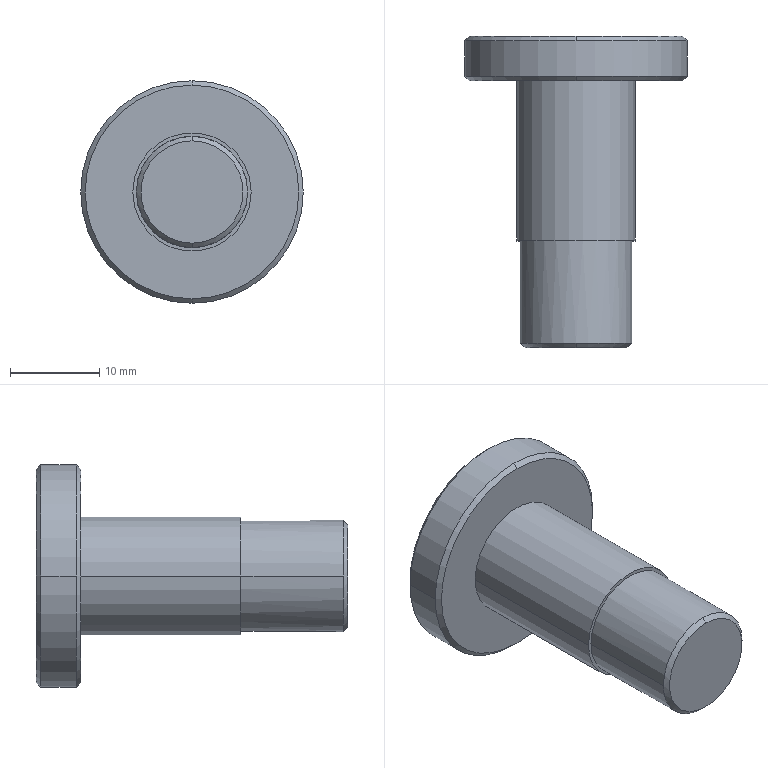Part | SolidWorks | features Chamfer 1, Revolution 1 | 1 solid | 16 faces | box 25 x 35 x 25 mm | volume 6404 mm3 | cone 6 | cylinder 6 | plane 4 | commonest cylinder face diameters 12.5 x2 13.3 x2 25 x2
STEP:
#1=CARTESIAN_POINT('',(-133.037,-447.686,-5.75));
#2=VERTEX_POINT('',#1);
#3=CARTESIAN_POINT('',(-133.037,-447.686,5.75));
#4=VERTEX_POINT('',#3);
#5=CARTESIAN_POINT('',(-133.037,-447.686,0.));
#6=DIRECTION('',(0.,-1.,0.));
#7=DIRECTION('',(1.,0.,0.));
#8=AXIS2_PLACEMENT_3D('',#5,#6,#7);
#9=CIRCLE('',#8,5.75);
#10=EDGE_CURVE('',#2,#4,#9,.T.);
#11=ORIENTED_EDGE('',*,*,#10,.F.);
#12=CARTESIAN_POINT('',(-133.037,-447.186,-6.25));
#13=VERTEX_POINT('',#12);
#14=CARTESIAN_POINT('',(-133.037,-447.186,-6.25));
#15=DIRECTION('',(0.,0.7071,-0.7071));
#16=VECTOR('',#15,1000.);
#17=LINE('',#14,#16);
#18=EDGE_CURVE('',#2,#13,#17,.T.);
#19=ORIENTED_EDGE('',*,*,#18,.T.);
#20=CARTESIAN_POINT('',(-126.787,-447.186,0.));
#21=VERTEX_POINT('',#20);
#22=CARTESIAN_POINT('',(-133.037,-447.186,0.));
#23=DIRECTION('',(0.,1.,0.));
#24=DIRECTION('',(0.,0.,-1.));
#25=AXIS2_PLACEMENT_3D('',#22,#23,#24);
#26=CIRCLE('',#25,6.25);
#27=EDGE_CURVE('',#21,#13,#26,.T.);
#28=ORIENTED_EDGE('',*,*,#27,.F.);
#29=CARTESIAN_POINT('',(-133.037,-447.186,6.25));
#30=VERTEX_POINT('',#29);
#31=CARTESIAN_POINT('',(-133.037,-447.186,0.));
#32=DIRECTION('',(0.,1.,0.));
#33=DIRECTION('',(0.,0.,-1.));
#34=AXIS2_PLACEMENT_3D('',#31,#32,#33);
#35=CIRCLE('',#34,6.25);
#36=EDGE_CURVE('',#30,#21,#35,.T.);
#37=ORIENTED_EDGE('',*,*,#36,.F.);
#38=CARTESIAN_POINT('',(-133.037,-447.186,6.25));
#39=DIRECTION('',(0.,0.7071,0.7071));
#40=VECTOR('',#39,1000.);
#41=LINE('',#38,#40);
#42=EDGE_CURVE('',#4,#30,#41,.T.);
#43=ORIENTED_EDGE('',*,*,#42,.F.);
#44=EDGE_LOOP('',(#11,#19,#28,#37,#43));
#45=FACE_OUTER_BOUND('',#44,.T.);
#46=CARTESIAN_POINT('',(-133.037,-447.186,0.));
#47=DIRECTION('',(0.,1.,0.));
#48=DIRECTION('',(0.,0.,1.));
#49=AXIS2_PLACEMENT_3D('',#46,#47,#48);
#50=CONICAL_SURFACE('',#49,6.25,0.7854);
#51=ADVANCED_FACE('',(#45),#50,.T.);
#52=CARTESIAN_POINT('',(-133.037,-417.686,-12.));
#53=VERTEX_POINT('',#52);
#54=CARTESIAN_POINT('',(-133.037,-417.686,12.));
#55=VERTEX_POINT('',#54);
#56=CARTESIAN_POINT('',(-133.037,-417.686,0.));
#57=DIRECTION('',(0.,-1.,0.));
#58=DIRECTION('',(1.,0.,0.));
#59=AXIS2_PLACEMENT_3D('',#56,#57,#58);
#60=CIRCLE('',#59,12.);
#61=EDGE_CURVE('',#53,#55,#60,.T.);
#62=ORIENTED_EDGE('',*,*,#61,.F.);
#63=CARTESIAN_POINT('',(-133.037,-417.186,-12.5));
#64=VERTEX_POINT('',#63);
#65=CARTESIAN_POINT('',(-133.037,-417.186,-12.5));
#66=DIRECTION('',(0.,0.7071,-0.7071));
#67=VECTOR('',#66,1000.);
#68=LINE('',#65,#67);
#69=EDGE_CURVE('',#53,#64,#68,.T.);
#70=ORIENTED_EDGE('',*,*,#69,.T.);
#71=CARTESIAN_POINT('',(-120.537,-417.186,0.));
#72=VERTEX_POINT('',#71);
#73=CARTESIAN_POINT('',(-133.037,-417.186,0.));
#74=DIRECTION('',(0.,1.,0.));
#75=DIRECTION('',(0.,0.,-1.));
#76=AXIS2_PLACEMENT_3D('',#73,#74,#75);
#77=CIRCLE('',#76,12.5);
#78=EDGE_CURVE('',#72,#64,#77,.T.);
#79=ORIENTED_EDGE('',*,*,#78,.F.);
#80=CARTESIAN_POINT('',(-133.037,-417.186,12.5));
#81=VERTEX_POINT('',#80);
#82=CARTESIAN_POINT('',(-133.037,-417.186,0.));
#83=DIRECTION('',(0.,1.,0.));
#84=DIRECTION('',(0.,0.,-1.));
#85=AXIS2_PLACEMENT_3D('',#82,#83,#84);
#86=CIRCLE('',#85,12.5);
#87=EDGE_CURVE('',#81,#72,#86,.T.);
#88=ORIENTED_EDGE('',*,*,#87,.F.);
#89=CARTESIAN_POINT('',(-133.037,-417.186,12.5));
#90=DIRECTION('',(0.,0.7071,0.7071));
#91=VECTOR('',#90,1000.);
#92=LINE('',#89,#91);
#93=EDGE_CURVE('',#55,#81,#92,.T.);
#94=ORIENTED_EDGE('',*,*,#93,.F.);
#95=EDGE_LOOP('',(#62,#70,#79,#88,#94));
#96=FACE_OUTER_BOUND('',#95,.T.);
#97=CARTESIAN_POINT('',(-133.037,-417.186,0.));
#98=DIRECTION('',(0.,1.,0.));
#99=DIRECTION('',(0.,0.,1.));
#100=AXIS2_PLACEMENT_3D('',#97,#98,#99);
#101=CONICAL_SURFACE('',#100,12.5,0.7854);
#102=ADVANCED_FACE('',(#96),#101,.T.);
#103=CARTESIAN_POINT('',(-133.037,-412.686,12.));
#104=VERTEX_POINT('',#103);
#105=CARTESIAN_POINT('',(-133.037,-412.686,-12.));
#106=VERTEX_POINT('',#105);
#107=CARTESIAN_POINT('',(-133.037,-412.686,0.));
#108=DIRECTION('',(0.,1.,0.));
#109=DIRECTION('',(-1.,0.,0.));
#110=AXIS2_PLACEMENT_3D('',#107,#108,#109);
#111=CIRCLE('',#110,12.);
#112=EDGE_CURVE('',#104,#106,#111,.T.);
#113=ORIENTED_EDGE('',*,*,#112,.F.);
#114=CARTESIAN_POINT('',(-133.037,-413.186,12.5));
#115=VERTEX_POINT('',#114);
#116=CARTESIAN_POINT('',(-133.037,-412.686,12.));
#117=DIRECTION('',(0.,-0.7071,0.7071));
#118=VECTOR('',#117,1000.);
#119=LINE('',#116,#118);
#120=EDGE_CURVE('',#104,#115,#119,.T.);
#121=ORIENTED_EDGE('',*,*,#120,.T.);
#122=CARTESIAN_POINT('',(-120.537,-413.186,0.));
#123=VERTEX_POINT('',#122);
#124=CARTESIAN_POINT('',(-133.037,-413.186,0.));
#125=DIRECTION('',(0.,-1.,0.));
#126=DIRECTION('',(0.,0.,1.));
#127=AXIS2_PLACEMENT_3D('',#124,#125,#126);
#128=CIRCLE('',#127,12.5);
#129=EDGE_CURVE('',#123,#115,#128,.T.);
#130=ORIENTED_EDGE('',*,*,#129,.F.);
#131=CARTESIAN_POINT('',(-133.037,-413.186,-12.5));
#132=VERTEX_POINT('',#131);
#133=CARTESIAN_POINT('',(-133.037,-413.186,0.));
#134=DIRECTION('',(0.,-1.,0.));
#135=DIRECTION('',(0.,0.,1.));
#136=AXIS2_PLACEMENT_3D('',#133,#134,#135);
#137=CIRCLE('',#136,12.5);
#138=EDGE_CURVE('',#132,#123,#137,.T.);
#139=ORIENTED_EDGE('',*,*,#138,.F.);
#140=CARTESIAN_POINT('',(-133.037,-412.686,-12.));
#141=DIRECTION('',(0.,-0.7071,-0.7071));
#142=VECTOR('',#141,1000.);
#143=LINE('',#140,#142);
#144=EDGE_CURVE('',#106,#132,#143,.T.);
#145=ORIENTED_EDGE('',*,*,#144,.F.);
#146=EDGE_LOOP('',(#113,#121,#130,#139,#145));
#147=FACE_OUTER_BOUND('',#146,.T.);
#148=CARTESIAN_POINT('',(-133.037,-412.686,0.));
#149=DIRECTION('',(0.,-1.,0.));
#150=DIRECTION('',(0.,0.,-1.));
#151=AXIS2_PLACEMENT_3D('',#148,#149,#150);
#152=CONICAL_SURFACE('',#151,12.,0.7854);
#153=ADVANCED_FACE('',(#147),#152,.T.);
#154=CARTESIAN_POINT('',(-145.537,-417.186,0.));
#155=VERTEX_POINT('',#154);
#156=CARTESIAN_POINT('',(-133.037,-417.186,0.));
#157=DIRECTION('',(0.,1.,0.));
#158=DIRECTION('',(0.,0.,-1.));
#159=AXIS2_PLACEMENT_3D('',#156,#157,#158);
#160=CIRCLE('',#159,12.5);
#161=EDGE_CURVE('',#155,#81,#160,.T.);
#162=ORIENTED_EDGE('',*,*,#161,.T.);
#163=ORIENTED_EDGE('',*,*,#87,.T.);
#164=CARTESIAN_POINT('',(-120.537,-412.686,0.));
#165=DIRECTION('',(0.,1.,0.));
#166=VECTOR('',#165,1000.);
#167=LINE('',#164,#166);
#168=EDGE_CURVE('',#72,#123,#167,.T.);
#169=ORIENTED_EDGE('',*,*,#168,.T.);
#170=ORIENTED_EDGE('',*,*,#129,.T.);
#171=CARTESIAN_POINT('',(-145.537,-413.186,0.));
#172=VERTEX_POINT('',#171);
#173=CARTESIAN_POINT('',(-133.037,-413.186,0.));
#174=DIRECTION('',(0.,-1.,0.));
#175=DIRECTION('',(0.,0.,1.));
#176=AXIS2_PLACEMENT_3D('',#173,#174,#175);
#177=CIRCLE('',#176,12.5);
#178=EDGE_CURVE('',#115,#172,#177,.T.);
#179=ORIENTED_EDGE('',*,*,#178,.T.);
#180=CARTESIAN_POINT('',(-145.537,-412.686,0.));
#181=DIRECTION('',(0.,1.,0.));
#182=VECTOR('',#181,1000.);
#183=LINE('',#180,#182);
#184=EDGE_CURVE('',#155,#172,#183,.T.);
#185=ORIENTED_EDGE('',*,*,#184,.F.);
#186=EDGE_LOOP('',(#162,#163,#169,#170,#179,#185));
#187=FACE_OUTER_BOUND('',#186,.T.);
#188=CARTESIAN_POINT('',(-133.037,-412.686,0.));
#189=DIRECTION('',(0.,1.,0.));
#190=DIRECTION('',(-1.,0.,0.));
#191=AXIS2_PLACEMENT_3D('',#188,#189,#190);
#192=CYLINDRICAL_SURFACE('',#191,12.5);
#193=ADVANCED_FACE('',(#187),#192,.T.);
#194=CARTESIAN_POINT('',(-139.687,-435.686,0.));
#195=VERTEX_POINT('',#194);
#196=CARTESIAN_POINT('',(-126.387,-435.686,0.));
#197=VERTEX_POINT('',#196);
#198=CARTESIAN_POINT('',(-133.037,-435.686,0.));
#199=DIRECTION('',(0.,1.,0.));
#200=DIRECTION('',(-1.,0.,0.));
#201=AXIS2_PLACEMENT_3D('',#198,#199,#200);
#202=CIRCLE('',#201,6.65);
#203=EDGE_CURVE('',#195,#197,#202,.T.);
#204=ORIENTED_EDGE('',*,*,#203,.T.);
#205=CARTESIAN_POINT('',(-126.387,-417.686,0.));
#206=VERTEX_POINT('',#205);
#207=CARTESIAN_POINT('',(-126.387,-412.686,0.));
#208=DIRECTION('',(0.,1.,0.));
#209=VECTOR('',#208,1000.);
#210=LINE('',#207,#209);
#211=EDGE_CURVE('',#197,#206,#210,.T.);
#212=ORIENTED_EDGE('',*,*,#211,.T.);
#213=CARTESIAN_POINT('',(-139.687,-417.686,0.));
#214=VERTEX_POINT('',#213);
#215=CARTESIAN_POINT('',(-133.037,-417.686,0.));
#216=DIRECTION('',(0.,1.,0.));
#217=DIRECTION('',(-1.,0.,0.));
#218=AXIS2_PLACEMENT_3D('',#215,#216,#217);
#219=CIRCLE('',#218,6.65);
#220=EDGE_CURVE('',#214,#206,#219,.T.);
#221=ORIENTED_EDGE('',*,*,#220,.F.);
#222=CARTESIAN_POINT('',(-139.687,-412.686,0.));
#223=DIRECTION('',(0.,1.,0.));
#224=VECTOR('',#223,1000.);
#225=LINE('',#222,#224);
#226=EDGE_CURVE('',#195,#214,#225,.T.);
#227=ORIENTED_EDGE('',*,*,#226,.F.);
#228=EDGE_LOOP('',(#204,#212,#221,#227));
#229=FACE_OUTER_BOUND('',#228,.T.);
#230=CARTESIAN_POINT('',(-133.037,-412.686,0.));
#231=DIRECTION('',(0.,1.,0.));
#232=DIRECTION('',(-1.,0.,0.));
#233=AXIS2_PLACEMENT_3D('',#230,#231,#232);
#234=CYLINDRICAL_SURFACE('',#233,6.65);
#235=ADVANCED_FACE('',(#229),#234,.T.);
#236=CARTESIAN_POINT('',(-139.287,-447.186,0.));
#237=VERTEX_POINT('',#236);
#238=CARTESIAN_POINT('',(-133.037,-447.186,0.));
#239=DIRECTION('',(0.,1.,0.));
#240=DIRECTION('',(0.,0.,-1.));
#241=AXIS2_PLACEMENT_3D('',#238,#239,#240);
#242=CIRCLE('',#241,6.25);
#243=EDGE_CURVE('',#237,#30,#242,.T.);
#244=ORIENTED_EDGE('',*,*,#243,.T.);
#245=ORIENTED_EDGE('',*,*,#36,.T.);
#246=CARTESIAN_POINT('',(-126.787,-435.686,0.));
#247=VERTEX_POINT('',#246);
#248=CARTESIAN_POINT('',(-126.787,-412.686,0.));
#249=DIRECTION('',(0.,1.,0.));
#250=VECTOR('',#249,1000.);
#251=LINE('',#248,#250);
#252=EDGE_CURVE('',#21,#247,#251,.T.);
#253=ORIENTED_EDGE('',*,*,#252,.T.);
#254=CARTESIAN_POINT('',(-139.287,-435.686,0.));
#255=VERTEX_POINT('',#254);
#256=CARTESIAN_POINT('',(-133.037,-435.686,0.));
#257=DIRECTION('',(0.,1.,0.));
#258=DIRECTION('',(-1.,0.,0.));
#259=AXIS2_PLACEMENT_3D('',#256,#257,#258);
#260=CIRCLE('',#259,6.25);
#261=EDGE_CURVE('',#255,#247,#260,.T.);
#262=ORIENTED_EDGE('',*,*,#261,.F.);
#263=CARTESIAN_POINT('',(-139.287,-412.686,0.));
#264=DIRECTION('',(0.,1.,0.));
#265=VECTOR('',#264,1000.);
#266=LINE('',#263,#265);
#267=EDGE_CURVE('',#237,#255,#266,.T.);
#268=ORIENTED_EDGE('',*,*,#267,.F.);
#269=EDGE_LOOP('',(#244,#245,#253,#262,#268));
#270=FACE_OUTER_BOUND('',#269,.T.);
#271=CARTESIAN_POINT('',(-133.037,-412.686,0.));
#272=DIRECTION('',(0.,1.,0.));
#273=DIRECTION('',(-1.,0.,0.));
#274=AXIS2_PLACEMENT_3D('',#271,#272,#273);
#275=CYLINDRICAL_SURFACE('',#274,6.25);
#276=ADVANCED_FACE('',(#270),#275,.T.);
#277=CARTESIAN_POINT('',(-133.037,-447.686,0.));
#278=DIRECTION('',(0.,-1.,0.));
#279=DIRECTION('',(1.,0.,0.));
#280=AXIS2_PLACEMENT_3D('',#277,#278,#279);
#281=CIRCLE('',#280,5.75);
#282=EDGE_CURVE('',#4,#2,#281,.T.);
#283=ORIENTED_EDGE('',*,*,#282,.T.);
#284=ORIENTED_EDGE('',*,*,#10,.T.);
#285=EDGE_LOOP('',(#283,#284));
#286=FACE_OUTER_BOUND('',#285,.T.);
#287=CARTESIAN_POINT('',(-139.287,-447.686,0.));
#288=DIRECTION('',(0.,-1.,0.));
#289=DIRECTION('',(1.,0.,0.));
#290=AXIS2_PLACEMENT_3D('',#287,#288,#289);
#291=PLANE('',#290);
#292=ADVANCED_FACE('',(#286),#291,.T.);
#293=ORIENTED_EDGE('',*,*,#252,.F.);
#294=ORIENTED_EDGE('',*,*,#27,.T.);
#295=CARTESIAN_POINT('',(-133.037,-447.186,0.));
#296=DIRECTION('',(0.,1.,0.));
#297=DIRECTION('',(0.,0.,-1.));
#298=AXIS2_PLACEMENT_3D('',#295,#296,#297);
#299=CIRCLE('',#298,6.25);
#300=EDGE_CURVE('',#13,#237,#299,.T.);
#301=ORIENTED_EDGE('',*,*,#300,.T.);
#302=ORIENTED_EDGE('',*,*,#267,.T.);
#303=CARTESIAN_POINT('',(-133.037,-435.686,0.));
#304=DIRECTION('',(0.,1.,0.));
#305=DIRECTION('',(-1.,0.,0.));
#306=AXIS2_PLACEMENT_3D('',#303,#304,#305);
#307=CIRCLE('',#306,6.25);
#308=EDGE_CURVE('',#247,#255,#307,.T.);
#309=ORIENTED_EDGE('',*,*,#308,.F.);
#310=EDGE_LOOP('',(#293,#294,#301,#302,#309));
#311=FACE_OUTER_BOUND('',#310,.T.);
#312=CARTESIAN_POINT('',(-133.037,-412.686,0.));
#313=DIRECTION('',(0.,1.,0.));
#314=DIRECTION('',(-1.,0.,0.));
#315=AXIS2_PLACEMENT_3D('',#312,#313,#314);
#316=CYLINDRICAL_SURFACE('',#315,6.25);
#317=ADVANCED_FACE('',(#311),#316,.T.);
#318=ORIENTED_EDGE('',*,*,#261,.T.);
#319=ORIENTED_EDGE('',*,*,#308,.T.);
#320=EDGE_LOOP('',(#318,#319));
#321=FACE_BOUND('',#320,.T.);
#322=ORIENTED_EDGE('',*,*,#203,.F.);
#323=CARTESIAN_POINT('',(-133.037,-435.686,0.));
#324=DIRECTION('',(0.,1.,0.));
#325=DIRECTION('',(-1.,0.,0.));
#326=AXIS2_PLACEMENT_3D('',#323,#324,#325);
#327=CIRCLE('',#326,6.65);
#328=EDGE_CURVE('',#197,#195,#327,.T.);
#329=ORIENTED_EDGE('',*,*,#328,.F.);
#330=EDGE_LOOP('',(#322,#329));
#331=FACE_OUTER_BOUND('',#330,.T.);
#332=CARTESIAN_POINT('',(-139.287,-435.686,0.));
#333=DIRECTION('',(0.,-1.,0.));
#334=DIRECTION('',(1.,0.,0.));
#335=AXIS2_PLACEMENT_3D('',#332,#333,#334);
#336=PLANE('',#335);
#337=ADVANCED_FACE('',(#321,#331),#336,.T.);
#338=ORIENTED_EDGE('',*,*,#211,.F.);
#339=ORIENTED_EDGE('',*,*,#328,.T.);
#340=ORIENTED_EDGE('',*,*,#226,.T.);
#341=CARTESIAN_POINT('',(-133.037,-417.686,0.));
#342=DIRECTION('',(0.,1.,0.));
#343=DIRECTION('',(-1.,0.,0.));
#344=AXIS2_PLACEMENT_3D('',#341,#342,#343);
#345=CIRCLE('',#344,6.65);
#346=EDGE_CURVE('',#206,#214,#345,.T.);
#347=ORIENTED_EDGE('',*,*,#346,.F.);
#348=EDGE_LOOP('',(#338,#339,#340,#347));
#349=FACE_OUTER_BOUND('',#348,.T.);
#350=CARTESIAN_POINT('',(-133.037,-412.686,0.));
#351=DIRECTION('',(0.,1.,0.));
#352=DIRECTION('',(-1.,0.,0.));
#353=AXIS2_PLACEMENT_3D('',#350,#351,#352);
#354=CYLINDRICAL_SURFACE('',#353,6.65);
#355=ADVANCED_FACE('',(#349),#354,.T.);
#356=CARTESIAN_POINT('',(-133.037,-417.686,0.));
#357=DIRECTION('',(0.,-1.,0.));
#358=DIRECTION('',(1.,0.,0.));
#359=AXIS2_PLACEMENT_3D('',#356,#357,#358);
#360=CIRCLE('',#359,12.);
#361=EDGE_CURVE('',#55,#53,#360,.T.);
#362=ORIENTED_EDGE('',*,*,#361,.T.);
#363=ORIENTED_EDGE('',*,*,#61,.T.);
#364=EDGE_LOOP('',(#362,#363));
#365=FACE_OUTER_BOUND('',#364,.T.);
#366=ORIENTED_EDGE('',*,*,#220,.T.);
#367=ORIENTED_EDGE('',*,*,#346,.T.);
#368=EDGE_LOOP('',(#366,#367));
#369=FACE_BOUND('',#368,.T.);
#370=CARTESIAN_POINT('',(-139.687,-417.686,0.));
#371=DIRECTION('',(0.,-1.,0.));
#372=DIRECTION('',(1.,0.,0.));
#373=AXIS2_PLACEMENT_3D('',#370,#371,#372);
#374=PLANE('',#373);
#375=ADVANCED_FACE('',(#365,#369),#374,.T.);
#376=ORIENTED_EDGE('',*,*,#168,.F.);
#377=ORIENTED_EDGE('',*,*,#78,.T.);
#378=CARTESIAN_POINT('',(-133.037,-417.186,0.));
#379=DIRECTION('',(0.,1.,0.));
#380=DIRECTION('',(0.,0.,-1.));
#381=AXIS2_PLACEMENT_3D('',#378,#379,#380);
#382=CIRCLE('',#381,12.5);
#383=EDGE_CURVE('',#64,#155,#382,.T.);
#384=ORIENTED_EDGE('',*,*,#383,.T.);
#385=ORIENTED_EDGE('',*,*,#184,.T.);
#386=CARTESIAN_POINT('',(-133.037,-413.186,0.));
#387=DIRECTION('',(0.,-1.,0.));
#388=DIRECTION('',(0.,0.,1.));
#389=AXIS2_PLACEMENT_3D('',#386,#387,#388);
#390=CIRCLE('',#389,12.5);
#391=EDGE_CURVE('',#172,#132,#390,.T.);
#392=ORIENTED_EDGE('',*,*,#391,.T.);
#393=ORIENTED_EDGE('',*,*,#138,.T.);
#394=EDGE_LOOP('',(#376,#377,#384,#385,#392,#393));
#395=FACE_OUTER_BOUND('',#394,.T.);
#396=CARTESIAN_POINT('',(-133.037,-412.686,0.));
#397=DIRECTION('',(0.,1.,0.));
#398=DIRECTION('',(-1.,0.,0.));
#399=AXIS2_PLACEMENT_3D('',#396,#397,#398);
#400=CYLINDRICAL_SURFACE('',#399,12.5);
#401=ADVANCED_FACE('',(#395),#400,.T.);
#402=CARTESIAN_POINT('',(-133.037,-412.686,0.));
#403=DIRECTION('',(0.,1.,0.));
#404=DIRECTION('',(-1.,0.,0.));
#405=AXIS2_PLACEMENT_3D('',#402,#403,#404);
#406=CIRCLE('',#405,12.);
#407=EDGE_CURVE('',#106,#104,#406,.T.);
#408=ORIENTED_EDGE('',*,*,#407,.T.);
#409=ORIENTED_EDGE('',*,*,#112,.T.);
#410=EDGE_LOOP('',(#408,#409));
#411=FACE_OUTER_BOUND('',#410,.T.);
#412=CARTESIAN_POINT('',(-145.537,-412.686,0.));
#413=DIRECTION('',(0.,1.,0.));
#414=DIRECTION('',(-1.,0.,0.));
#415=AXIS2_PLACEMENT_3D('',#412,#413,#414);
#416=PLANE('',#415);
#417=ADVANCED_FACE('',(#411),#416,.T.);
#418=ORIENTED_EDGE('',*,*,#120,.F.);
#419=ORIENTED_EDGE('',*,*,#407,.F.);
#420=ORIENTED_EDGE('',*,*,#144,.T.);
#421=ORIENTED_EDGE('',*,*,#391,.F.);
#422=ORIENTED_EDGE('',*,*,#178,.F.);
#423=EDGE_LOOP('',(#418,#419,#420,#421,#422));
#424=FACE_OUTER_BOUND('',#423,.T.);
#425=CARTESIAN_POINT('',(-133.037,-412.686,0.));
#426=DIRECTION('',(0.,-1.,0.));
#427=DIRECTION('',(0.,0.,-1.));
#428=AXIS2_PLACEMENT_3D('',#425,#426,#427);
#429=CONICAL_SURFACE('',#428,12.,0.7854);
#430=ADVANCED_FACE('',(#424),#429,.T.);
#431=ORIENTED_EDGE('',*,*,#69,.F.);
#432=ORIENTED_EDGE('',*,*,#361,.F.);
#433=ORIENTED_EDGE('',*,*,#93,.T.);
#434=ORIENTED_EDGE('',*,*,#161,.F.);
#435=ORIENTED_EDGE('',*,*,#383,.F.);
#436=EDGE_LOOP('',(#431,#432,#433,#434,#435));
#437=FACE_OUTER_BOUND('',#436,.T.);
#438=CARTESIAN_POINT('',(-133.037,-417.186,0.));
#439=DIRECTION('',(0.,1.,0.));
#440=DIRECTION('',(0.,0.,1.));
#441=AXIS2_PLACEMENT_3D('',#438,#439,#440);
#442=CONICAL_SURFACE('',#441,12.5,0.7854);
#443=ADVANCED_FACE('',(#437),#442,.T.);
#444=ORIENTED_EDGE('',*,*,#18,.F.);
#445=ORIENTED_EDGE('',*,*,#282,.F.);
#446=ORIENTED_EDGE('',*,*,#42,.T.);
#447=ORIENTED_EDGE('',*,*,#243,.F.);
#448=ORIENTED_EDGE('',*,*,#300,.F.);
#449=EDGE_LOOP('',(#444,#445,#446,#447,#448));
#450=FACE_OUTER_BOUND('',#449,.T.);
#451=CARTESIAN_POINT('',(-133.037,-447.186,0.));
#452=DIRECTION('',(0.,1.,0.));
#453=DIRECTION('',(0.,0.,1.));
#454=AXIS2_PLACEMENT_3D('',#451,#452,#453);
#455=CONICAL_SURFACE('',#454,6.25,0.7854);
#456=ADVANCED_FACE('',(#450),#455,.T.);
#457=CLOSED_SHELL('',(#51,#102,#153,#193,#235,#276,#292,#317,#337,#355,#375,#401,#417,#430,#443,#456));
#458=MANIFOLD_SOLID_BREP('',#457);
#459=CARTESIAN_POINT('',(0.,0.,0.));
#460=DIRECTION('',(0.,0.,1.));
#461=DIRECTION('',(1.,0.,0.));
#462=AXIS2_PLACEMENT_3D('',#459,#460,#461);
#463=(LENGTH_UNIT()NAMED_UNIT(*)SI_UNIT(.MILLI.,.METRE.));
#464=UNCERTAINTY_MEASURE_WITH_UNIT(LENGTH_MEASURE(0.00001),#463,'','');
#465=(NAMED_UNIT(*)PLANE_ANGLE_UNIT()SI_UNIT($,.RADIAN.));
#466=(NAMED_UNIT(*)SI_UNIT($,.STERADIAN.)SOLID_ANGLE_UNIT());
#467=(GEOMETRIC_REPRESENTATION_CONTEXT(3)GLOBAL_UNCERTAINTY_ASSIGNED_CONTEXT((#464))GLOBAL_UNIT_ASSIGNED_CONTEXT((#463,#465,#466))REPRESENTATION_CONTEXT('',''));
#468=ADVANCED_BREP_SHAPE_REPRESENTATION('',(#458,#462),#467);